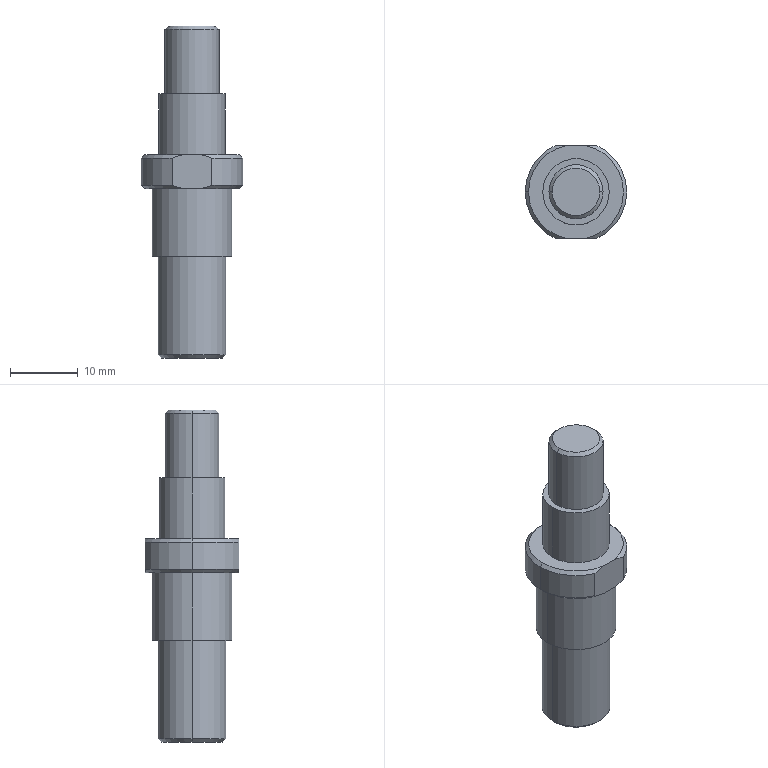Part | SolidWorks | features ICE 5, Chamfer 1, Extrusion 1 | 1 solid | 29 faces | box 15 x 13.8 x 49 mm | volume 4297 mm3 | cylinder 11 | cone 10 | plane 8 | commonest cylinder face diameters 15 x3 8 x2 9.8 x2 10 x2 11.8 x2
STEP:
#1=CARTESIAN_POINT('',(-4.5,0.,-24.5));
#2=VERTEX_POINT('',#1);
#3=CARTESIAN_POINT('',(4.5,0.,-24.5));
#4=VERTEX_POINT('',#3);
#5=CARTESIAN_POINT('',(0.,0.,-24.5));
#6=DIRECTION('',(0.,0.,-1.));
#7=DIRECTION('',(1.,0.,0.));
#8=AXIS2_PLACEMENT_3D('',#5,#6,#7);
#9=CIRCLE('',#8,4.5);
#10=EDGE_CURVE('',#2,#4,#9,.T.);
#11=ORIENTED_EDGE('',*,*,#10,.F.);
#12=CARTESIAN_POINT('',(-5.,0.,-24.));
#13=VERTEX_POINT('',#12);
#14=CARTESIAN_POINT('',(-4.5,0.,-24.5));
#15=DIRECTION('',(-0.7071,0.,0.7071));
#16=VECTOR('',#15,1000.);
#17=LINE('',#14,#16);
#18=EDGE_CURVE('',#2,#13,#17,.T.);
#19=ORIENTED_EDGE('',*,*,#18,.T.);
#20=CARTESIAN_POINT('',(5.,0.,-24.));
#21=VERTEX_POINT('',#20);
#22=CARTESIAN_POINT('',(0.,0.,-24.));
#23=DIRECTION('',(0.,0.,1.));
#24=DIRECTION('',(1.,0.,0.));
#25=AXIS2_PLACEMENT_3D('',#22,#23,#24);
#26=CIRCLE('',#25,5.);
#27=EDGE_CURVE('',#21,#13,#26,.T.);
#28=ORIENTED_EDGE('',*,*,#27,.F.);
#29=CARTESIAN_POINT('',(4.5,0.,-24.5));
#30=DIRECTION('',(0.7071,0.,0.7071));
#31=VECTOR('',#30,1000.);
#32=LINE('',#29,#31);
#33=EDGE_CURVE('',#4,#21,#32,.T.);
#34=ORIENTED_EDGE('',*,*,#33,.F.);
#35=EDGE_LOOP('',(#11,#19,#28,#34));
#36=FACE_OUTER_BOUND('',#35,.T.);
#37=CARTESIAN_POINT('',(0.,0.,-24.5));
#38=DIRECTION('',(0.,0.,1.));
#39=DIRECTION('',(1.,0.,0.));
#40=AXIS2_PLACEMENT_3D('',#37,#38,#39);
#41=CONICAL_SURFACE('',#40,4.5,0.7854);
#42=ADVANCED_FACE('',(#36),#41,.T.);
#43=CARTESIAN_POINT('',(3.5,0.,24.5));
#44=VERTEX_POINT('',#43);
#45=CARTESIAN_POINT('',(-3.5,0.,24.5));
#46=VERTEX_POINT('',#45);
#47=CARTESIAN_POINT('',(0.,0.,24.5));
#48=DIRECTION('',(0.,0.,1.));
#49=DIRECTION('',(1.,0.,0.));
#50=AXIS2_PLACEMENT_3D('',#47,#48,#49);
#51=CIRCLE('',#50,3.5);
#52=EDGE_CURVE('',#44,#46,#51,.T.);
#53=ORIENTED_EDGE('',*,*,#52,.F.);
#54=CARTESIAN_POINT('',(4.,0.,24.));
#55=VERTEX_POINT('',#54);
#56=CARTESIAN_POINT('',(3.5,0.,24.5));
#57=DIRECTION('',(0.7071,0.,-0.7071));
#58=VECTOR('',#57,1000.);
#59=LINE('',#56,#58);
#60=EDGE_CURVE('',#44,#55,#59,.T.);
#61=ORIENTED_EDGE('',*,*,#60,.T.);
#62=CARTESIAN_POINT('',(-4.,0.,24.));
#63=VERTEX_POINT('',#62);
#64=CARTESIAN_POINT('',(0.,0.,24.));
#65=DIRECTION('',(0.,0.,-1.));
#66=DIRECTION('',(1.,0.,0.));
#67=AXIS2_PLACEMENT_3D('',#64,#65,#66);
#68=CIRCLE('',#67,4.);
#69=EDGE_CURVE('',#63,#55,#68,.T.);
#70=ORIENTED_EDGE('',*,*,#69,.F.);
#71=CARTESIAN_POINT('',(-3.5,0.,24.5));
#72=DIRECTION('',(-0.7071,0.,-0.7071));
#73=VECTOR('',#72,1000.);
#74=LINE('',#71,#73);
#75=EDGE_CURVE('',#46,#63,#74,.T.);
#76=ORIENTED_EDGE('',*,*,#75,.F.);
#77=EDGE_LOOP('',(#53,#61,#70,#76));
#78=FACE_OUTER_BOUND('',#77,.T.);
#79=CARTESIAN_POINT('',(0.,0.,24.5));
#80=DIRECTION('',(0.,0.,-1.));
#81=DIRECTION('',(-1.,0.,0.));
#82=AXIS2_PLACEMENT_3D('',#79,#80,#81);
#83=CONICAL_SURFACE('',#82,3.5,0.7854);
#84=ADVANCED_FACE('',(#78),#83,.T.);
#85=CARTESIAN_POINT('',(-7.,0.,5.5));
#86=VERTEX_POINT('',#85);
#87=CARTESIAN_POINT('',(-1.179,-6.9,5.5));
#88=VERTEX_POINT('',#87);
#89=CARTESIAN_POINT('',(0.,0.,5.5));
#90=DIRECTION('',(0.,0.,1.));
#91=DIRECTION('',(1.,0.,0.));
#92=AXIS2_PLACEMENT_3D('',#89,#90,#91);
#93=CIRCLE('',#92,7.);
#94=EDGE_CURVE('',#86,#88,#93,.T.);
#95=ORIENTED_EDGE('',*,*,#94,.F.);
#96=CARTESIAN_POINT('',(-7.5,0.,5.));
#97=VERTEX_POINT('',#96);
#98=CARTESIAN_POINT('',(-7.,0.,5.5));
#99=DIRECTION('',(-0.7071,0.,-0.7071));
#100=VECTOR('',#99,1000.);
#101=LINE('',#98,#100);
#102=EDGE_CURVE('',#86,#97,#101,.T.);
#103=ORIENTED_EDGE('',*,*,#102,.T.);
#104=CARTESIAN_POINT('',(-2.939,-6.9,5.));
#105=VERTEX_POINT('',#104);
#106=CARTESIAN_POINT('',(0.,0.,5.));
#107=DIRECTION('',(0.,0.,-1.));
#108=DIRECTION('',(1.,0.,0.));
#109=AXIS2_PLACEMENT_3D('',#106,#107,#108);
#110=CIRCLE('',#109,7.5);
#111=EDGE_CURVE('',#105,#97,#110,.T.);
#112=ORIENTED_EDGE('',*,*,#111,.F.);
#113=CARTESIAN_POINT('',(-1.179,-6.9,5.5));
#114=CARTESIAN_POINT('',(-1.782,-6.9,5.398));
#115=CARTESIAN_POINT('',(-2.367,-6.9,5.224));
#116=CARTESIAN_POINT('',(-2.939,-6.9,5.));
#117=B_SPLINE_CURVE_WITH_KNOTS('',3,(#113,#114,#115,#116),.UNSPECIFIED.,.F.,.F.,(4,4),(0.01931,0.02115),.UNSPECIFIED.);
#118=EDGE_CURVE('',#88,#105,#117,.T.);
#119=ORIENTED_EDGE('',*,*,#118,.F.);
#120=EDGE_LOOP('',(#95,#103,#112,#119));
#121=FACE_OUTER_BOUND('',#120,.T.);
#122=CARTESIAN_POINT('',(0.,0.,5.5));
#123=DIRECTION('',(0.,0.,-1.));
#124=DIRECTION('',(-1.,0.,0.));
#125=AXIS2_PLACEMENT_3D('',#122,#123,#124);
#126=CONICAL_SURFACE('',#125,7.,0.7854);
#127=ADVANCED_FACE('',(#121),#126,.T.);
#128=CARTESIAN_POINT('',(7.,0.,0.5));
#129=VERTEX_POINT('',#128);
#130=CARTESIAN_POINT('',(1.179,-6.9,0.5));
#131=VERTEX_POINT('',#130);
#132=CARTESIAN_POINT('',(0.,0.,0.5));
#133=DIRECTION('',(0.,0.,-1.));
#134=DIRECTION('',(-1.,0.,0.));
#135=AXIS2_PLACEMENT_3D('',#132,#133,#134);
#136=CIRCLE('',#135,7.);
#137=EDGE_CURVE('',#129,#131,#136,.T.);
#138=ORIENTED_EDGE('',*,*,#137,.F.);
#139=CARTESIAN_POINT('',(7.5,0.,1.));
#140=VERTEX_POINT('',#139);
#141=CARTESIAN_POINT('',(7.,0.,0.5));
#142=DIRECTION('',(0.7071,0.,0.7071));
#143=VECTOR('',#142,1000.);
#144=LINE('',#141,#143);
#145=EDGE_CURVE('',#129,#140,#144,.T.);
#146=ORIENTED_EDGE('',*,*,#145,.T.);
#147=CARTESIAN_POINT('',(2.939,-6.9,1.));
#148=VERTEX_POINT('',#147);
#149=CARTESIAN_POINT('',(0.,0.,1.));
#150=DIRECTION('',(0.,0.,1.));
#151=DIRECTION('',(-1.,0.,0.));
#152=AXIS2_PLACEMENT_3D('',#149,#150,#151);
#153=CIRCLE('',#152,7.5);
#154=EDGE_CURVE('',#148,#140,#153,.T.);
#155=ORIENTED_EDGE('',*,*,#154,.F.);
#156=CARTESIAN_POINT('',(1.179,-6.9,0.5));
#157=CARTESIAN_POINT('',(1.782,-6.9,0.6016));
#158=CARTESIAN_POINT('',(2.367,-6.9,0.7758));
#159=CARTESIAN_POINT('',(2.939,-6.9,1.));
#160=B_SPLINE_CURVE_WITH_KNOTS('',3,(#156,#157,#158,#159),.UNSPECIFIED.,.F.,.F.,(4,4),(0.01931,0.02115),.UNSPECIFIED.);
#161=EDGE_CURVE('',#131,#148,#160,.T.);
#162=ORIENTED_EDGE('',*,*,#161,.F.);
#163=EDGE_LOOP('',(#138,#146,#155,#162));
#164=FACE_OUTER_BOUND('',#163,.T.);
#165=CARTESIAN_POINT('',(0.,0.,0.5));
#166=DIRECTION('',(0.,0.,1.));
#167=DIRECTION('',(1.,0.,0.));
#168=AXIS2_PLACEMENT_3D('',#165,#166,#167);
#169=CONICAL_SURFACE('',#168,7.,0.7854);
#170=ADVANCED_FACE('',(#164),#169,.T.);
#171=CARTESIAN_POINT('',(-5.,0.,-9.5));
#172=VERTEX_POINT('',#171);
#173=CARTESIAN_POINT('',(5.,0.,-9.5));
#174=VERTEX_POINT('',#173);
#175=CARTESIAN_POINT('',(0.,0.,-9.5));
#176=DIRECTION('',(0.,0.,-1.));
#177=DIRECTION('',(-1.,0.,0.));
#178=AXIS2_PLACEMENT_3D('',#175,#176,#177);
#179=CIRCLE('',#178,5.);
#180=EDGE_CURVE('',#172,#174,#179,.T.);
#181=ORIENTED_EDGE('',*,*,#180,.T.);
#182=CARTESIAN_POINT('',(5.,0.,-9.5));
#183=DIRECTION('',(0.,0.,-1.));
#184=VECTOR('',#183,1000.);
#185=LINE('',#182,#184);
#186=EDGE_CURVE('',#174,#21,#185,.T.);
#187=ORIENTED_EDGE('',*,*,#186,.T.);
#188=ORIENTED_EDGE('',*,*,#27,.T.);
#189=CARTESIAN_POINT('',(-5.,0.,-9.5));
#190=DIRECTION('',(0.,0.,-1.));
#191=VECTOR('',#190,1000.);
#192=LINE('',#189,#191);
#193=EDGE_CURVE('',#172,#13,#192,.T.);
#194=ORIENTED_EDGE('',*,*,#193,.F.);
#195=EDGE_LOOP('',(#181,#187,#188,#194));
#196=FACE_OUTER_BOUND('',#195,.T.);
#197=CARTESIAN_POINT('',(0.,0.,-9.5));
#198=DIRECTION('',(0.,0.,-1.));
#199=DIRECTION('',(-1.,0.,0.));
#200=AXIS2_PLACEMENT_3D('',#197,#198,#199);
#201=CYLINDRICAL_SURFACE('',#200,5.);
#202=ADVANCED_FACE('',(#196),#201,.T.);
#203=CARTESIAN_POINT('',(4.,0.,14.5));
#204=VERTEX_POINT('',#203);
#205=CARTESIAN_POINT('',(-4.,0.,14.5));
#206=VERTEX_POINT('',#205);
#207=CARTESIAN_POINT('',(0.,0.,14.5));
#208=DIRECTION('',(0.,0.,1.));
#209=DIRECTION('',(1.,0.,0.));
#210=AXIS2_PLACEMENT_3D('',#207,#208,#209);
#211=CIRCLE('',#210,4.);
#212=EDGE_CURVE('',#204,#206,#211,.T.);
#213=ORIENTED_EDGE('',*,*,#212,.T.);
#214=CARTESIAN_POINT('',(-4.,0.,14.5));
#215=DIRECTION('',(0.,0.,1.));
#216=VECTOR('',#215,1000.);
#217=LINE('',#214,#216);
#218=EDGE_CURVE('',#206,#63,#217,.T.);
#219=ORIENTED_EDGE('',*,*,#218,.T.);
#220=ORIENTED_EDGE('',*,*,#69,.T.);
#221=CARTESIAN_POINT('',(4.,0.,14.5));
#222=DIRECTION('',(0.,0.,1.));
#223=VECTOR('',#222,1000.);
#224=LINE('',#221,#223);
#225=EDGE_CURVE('',#204,#55,#224,.T.);
#226=ORIENTED_EDGE('',*,*,#225,.F.);
#227=EDGE_LOOP('',(#213,#219,#220,#226));
#228=FACE_OUTER_BOUND('',#227,.T.);
#229=CARTESIAN_POINT('',(0.,0.,14.5));
#230=DIRECTION('',(0.,0.,1.));
#231=DIRECTION('',(1.,0.,0.));
#232=AXIS2_PLACEMENT_3D('',#229,#230,#231);
#233=CYLINDRICAL_SURFACE('',#232,4.);
#234=ADVANCED_FACE('',(#228),#233,.T.);
#235=CARTESIAN_POINT('',(4.9,0.,5.5));
#236=VERTEX_POINT('',#235);
#237=CARTESIAN_POINT('',(-4.9,0.,5.5));
#238=VERTEX_POINT('',#237);
#239=CARTESIAN_POINT('',(0.,0.,5.5));
#240=DIRECTION('',(0.,0.,1.));
#241=DIRECTION('',(1.,0.,0.));
#242=AXIS2_PLACEMENT_3D('',#239,#240,#241);
#243=CIRCLE('',#242,4.9);
#244=EDGE_CURVE('',#236,#238,#243,.T.);
#245=ORIENTED_EDGE('',*,*,#244,.T.);
#246=CARTESIAN_POINT('',(-4.9,0.,14.5));
#247=VERTEX_POINT('',#246);
#248=CARTESIAN_POINT('',(-4.9,0.,5.5));
#249=DIRECTION('',(0.,0.,1.));
#250=VECTOR('',#249,1000.);
#251=LINE('',#248,#250);
#252=EDGE_CURVE('',#238,#247,#251,.T.);
#253=ORIENTED_EDGE('',*,*,#252,.T.);
#254=CARTESIAN_POINT('',(4.9,0.,14.5));
#255=VERTEX_POINT('',#254);
#256=CARTESIAN_POINT('',(0.,0.,14.5));
#257=DIRECTION('',(0.,0.,-1.));
#258=DIRECTION('',(1.,0.,0.));
#259=AXIS2_PLACEMENT_3D('',#256,#257,#258);
#260=CIRCLE('',#259,4.9);
#261=EDGE_CURVE('',#247,#255,#260,.T.);
#262=ORIENTED_EDGE('',*,*,#261,.T.);
#263=CARTESIAN_POINT('',(4.9,0.,5.5));
#264=DIRECTION('',(0.,0.,1.));
#265=VECTOR('',#264,1000.);
#266=LINE('',#263,#265);
#267=EDGE_CURVE('',#236,#255,#266,.T.);
#268=ORIENTED_EDGE('',*,*,#267,.F.);
#269=EDGE_LOOP('',(#245,#253,#262,#268));
#270=FACE_OUTER_BOUND('',#269,.T.);
#271=CARTESIAN_POINT('',(0.,0.,5.5));
#272=DIRECTION('',(0.,0.,1.));
#273=DIRECTION('',(1.,0.,0.));
#274=AXIS2_PLACEMENT_3D('',#271,#272,#273);
#275=CYLINDRICAL_SURFACE('',#274,4.9);
#276=ADVANCED_FACE('',(#270),#275,.T.);
#277=ORIENTED_EDGE('',*,*,#111,.T.);
#278=CARTESIAN_POINT('',(-7.5,0.,1.));
#279=VERTEX_POINT('',#278);
#280=CARTESIAN_POINT('',(-7.5,0.,24.5));
#281=DIRECTION('',(0.,0.,-1.));
#282=VECTOR('',#281,1000.);
#283=LINE('',#280,#282);
#284=EDGE_CURVE('',#97,#279,#283,.T.);
#285=ORIENTED_EDGE('',*,*,#284,.T.);
#286=CARTESIAN_POINT('',(-2.939,-6.9,1.));
#287=VERTEX_POINT('',#286);
#288=CARTESIAN_POINT('',(0.,0.,1.));
#289=DIRECTION('',(0.,0.,1.));
#290=DIRECTION('',(-1.,0.,0.));
#291=AXIS2_PLACEMENT_3D('',#288,#289,#290);
#292=CIRCLE('',#291,7.5);
#293=EDGE_CURVE('',#279,#287,#292,.T.);
#294=ORIENTED_EDGE('',*,*,#293,.T.);
#295=CARTESIAN_POINT('',(-2.939,-6.9,24.5));
#296=DIRECTION('',(0.,0.,1.));
#297=VECTOR('',#296,1000.);
#298=LINE('',#295,#297);
#299=EDGE_CURVE('',#287,#105,#298,.T.);
#300=ORIENTED_EDGE('',*,*,#299,.T.);
#301=EDGE_LOOP('',(#277,#285,#294,#300));
#302=FACE_OUTER_BOUND('',#301,.T.);
#303=CARTESIAN_POINT('',(0.,0.,24.5));
#304=DIRECTION('',(0.,0.,-1.));
#305=DIRECTION('',(-1.,0.,0.));
#306=AXIS2_PLACEMENT_3D('',#303,#304,#305);
#307=CYLINDRICAL_SURFACE('',#306,7.5);
#308=ADVANCED_FACE('',(#302),#307,.T.);
#309=CARTESIAN_POINT('',(-5.9,0.,0.5));
#310=VERTEX_POINT('',#309);
#311=CARTESIAN_POINT('',(5.9,0.,0.5));
#312=VERTEX_POINT('',#311);
#313=CARTESIAN_POINT('',(0.,0.,0.5));
#314=DIRECTION('',(0.,0.,-1.));
#315=DIRECTION('',(-1.,0.,0.));
#316=AXIS2_PLACEMENT_3D('',#313,#314,#315);
#317=CIRCLE('',#316,5.9);
#318=EDGE_CURVE('',#310,#312,#317,.T.);
#319=ORIENTED_EDGE('',*,*,#318,.T.);
#320=CARTESIAN_POINT('',(5.9,0.,-9.5));
#321=VERTEX_POINT('',#320);
#322=CARTESIAN_POINT('',(5.9,0.,0.5));
#323=DIRECTION('',(0.,0.,-1.));
#324=VECTOR('',#323,1000.);
#325=LINE('',#322,#324);
#326=EDGE_CURVE('',#312,#321,#325,.T.);
#327=ORIENTED_EDGE('',*,*,#326,.T.);
#328=CARTESIAN_POINT('',(-5.9,0.,-9.5));
#329=VERTEX_POINT('',#328);
#330=CARTESIAN_POINT('',(0.,0.,-9.5));
#331=DIRECTION('',(0.,0.,1.));
#332=DIRECTION('',(-1.,0.,0.));
#333=AXIS2_PLACEMENT_3D('',#330,#331,#332);
#334=CIRCLE('',#333,5.9);
#335=EDGE_CURVE('',#321,#329,#334,.T.);
#336=ORIENTED_EDGE('',*,*,#335,.T.);
#337=CARTESIAN_POINT('',(-5.9,0.,0.5));
#338=DIRECTION('',(0.,0.,-1.));
#339=VECTOR('',#338,1000.);
#340=LINE('',#337,#339);
#341=EDGE_CURVE('',#310,#329,#340,.T.);
#342=ORIENTED_EDGE('',*,*,#341,.F.);
#343=EDGE_LOOP('',(#319,#327,#336,#342));
#344=FACE_OUTER_BOUND('',#343,.T.);
#345=CARTESIAN_POINT('',(0.,0.,0.5));
#346=DIRECTION('',(0.,0.,-1.));
#347=DIRECTION('',(-1.,0.,0.));
#348=AXIS2_PLACEMENT_3D('',#345,#346,#347);
#349=CYLINDRICAL_SURFACE('',#348,5.9);
#350=ADVANCED_FACE('',(#344),#349,.T.);
#351=CARTESIAN_POINT('',(2.939,6.9,5.));
#352=VERTEX_POINT('',#351);
#353=CARTESIAN_POINT('',(2.939,-6.9,5.));
#354=VERTEX_POINT('',#353);
#355=CARTESIAN_POINT('',(0.,0.,5.));
#356=DIRECTION('',(0.,0.,-1.));
#357=DIRECTION('',(1.,0.,0.));
#358=AXIS2_PLACEMENT_3D('',#355,#356,#357);
#359=CIRCLE('',#358,7.5);
#360=EDGE_CURVE('',#352,#354,#359,.T.);
#361=ORIENTED_EDGE('',*,*,#360,.T.);
#362=CARTESIAN_POINT('',(2.939,-6.9,24.5));
#363=DIRECTION('',(0.,0.,-1.));
#364=VECTOR('',#363,1000.);
#365=LINE('',#362,#364);
#366=EDGE_CURVE('',#354,#148,#365,.T.);
#367=ORIENTED_EDGE('',*,*,#366,.T.);
#368=ORIENTED_EDGE('',*,*,#154,.T.);
#369=CARTESIAN_POINT('',(2.939,6.9,1.));
#370=VERTEX_POINT('',#369);
#371=CARTESIAN_POINT('',(0.,0.,1.));
#372=DIRECTION('',(0.,0.,1.));
#373=DIRECTION('',(-1.,0.,0.));
#374=AXIS2_PLACEMENT_3D('',#371,#372,#373);
#375=CIRCLE('',#374,7.5);
#376=EDGE_CURVE('',#140,#370,#375,.T.);
#377=ORIENTED_EDGE('',*,*,#376,.T.);
#378=CARTESIAN_POINT('',(2.939,6.9,24.5));
#379=DIRECTION('',(0.,0.,1.));
#380=VECTOR('',#379,1000.);
#381=LINE('',#378,#380);
#382=EDGE_CURVE('',#370,#352,#381,.T.);
#383=ORIENTED_EDGE('',*,*,#382,.T.);
#384=EDGE_LOOP('',(#361,#367,#368,#377,#383));
#385=FACE_OUTER_BOUND('',#384,.T.);
#386=CARTESIAN_POINT('',(0.,0.,24.5));
#387=DIRECTION('',(0.,0.,-1.));
#388=DIRECTION('',(-1.,0.,0.));
#389=AXIS2_PLACEMENT_3D('',#386,#387,#388);
#390=CYLINDRICAL_SURFACE('',#389,7.5);
#391=ADVANCED_FACE('',(#385),#390,.T.);
#392=CARTESIAN_POINT('',(-1.179,-6.9,0.5));
#393=VERTEX_POINT('',#392);
#394=CARTESIAN_POINT('',(-2.939,-6.9,1.));
#395=CARTESIAN_POINT('',(-2.656,-6.9,0.889));
#396=CARTESIAN_POINT('',(-2.368,-6.9,0.7896));
#397=CARTESIAN_POINT('',(-1.78,-6.9,0.6203));
#398=CARTESIAN_POINT('',(-1.479,-6.9,0.5506));
#399=CARTESIAN_POINT('',(-1.179,-6.9,0.5));
#400=B_SPLINE_CURVE_WITH_KNOTS('',3,(#394,#395,#396,#397,#398,#399),.UNSPECIFIED.,.F.,.F.,(4,2,4),(0.01512,0.01603,0.01694),.UNSPECIFIED.);
#401=EDGE_CURVE('',#287,#393,#400,.T.);
#402=ORIENTED_EDGE('',*,*,#401,.F.);
#403=ORIENTED_EDGE('',*,*,#293,.F.);
#404=CARTESIAN_POINT('',(-2.939,6.9,1.));
#405=VERTEX_POINT('',#404);
#406=CARTESIAN_POINT('',(0.,0.,1.));
#407=DIRECTION('',(0.,0.,1.));
#408=DIRECTION('',(-1.,0.,0.));
#409=AXIS2_PLACEMENT_3D('',#406,#407,#408);
#410=CIRCLE('',#409,7.5);
#411=EDGE_CURVE('',#405,#279,#410,.T.);
#412=ORIENTED_EDGE('',*,*,#411,.F.);
#413=CARTESIAN_POINT('',(-1.179,6.9,0.5));
#414=VERTEX_POINT('',#413);
#415=CARTESIAN_POINT('',(-1.179,6.9,0.5));
#416=CARTESIAN_POINT('',(-1.782,6.9,0.6016));
#417=CARTESIAN_POINT('',(-2.367,6.9,0.7758));
#418=CARTESIAN_POINT('',(-2.939,6.9,1.));
#419=B_SPLINE_CURVE_WITH_KNOTS('',3,(#415,#416,#417,#418),.UNSPECIFIED.,.F.,.F.,(4,4),(0.01931,0.02115),.UNSPECIFIED.);
#420=EDGE_CURVE('',#414,#405,#419,.T.);
#421=ORIENTED_EDGE('',*,*,#420,.F.);
#422=CARTESIAN_POINT('',(0.,0.,0.5));
#423=DIRECTION('',(0.,0.,-1.));
#424=DIRECTION('',(-1.,0.,0.));
#425=AXIS2_PLACEMENT_3D('',#422,#423,#424);
#426=CIRCLE('',#425,7.);
#427=EDGE_CURVE('',#393,#414,#426,.T.);
#428=ORIENTED_EDGE('',*,*,#427,.F.);
#429=EDGE_LOOP('',(#402,#403,#412,#421,#428));
#430=FACE_OUTER_BOUND('',#429,.T.);
#431=CARTESIAN_POINT('',(0.,0.,0.5));
#432=DIRECTION('',(0.,0.,1.));
#433=DIRECTION('',(1.,0.,0.));
#434=AXIS2_PLACEMENT_3D('',#431,#432,#433);
#435=CONICAL_SURFACE('',#434,7.,0.7854);
#436=ADVANCED_FACE('',(#430),#435,.T.);
#437=CARTESIAN_POINT('',(1.179,-6.9,5.5));
#438=VERTEX_POINT('',#437);
#439=CARTESIAN_POINT('',(2.939,-6.9,5.));
#440=CARTESIAN_POINT('',(2.656,-6.9,5.111));
#441=CARTESIAN_POINT('',(2.368,-6.9,5.21));
#442=CARTESIAN_POINT('',(1.78,-6.9,5.38));
#443=CARTESIAN_POINT('',(1.479,-6.9,5.449));
#444=CARTESIAN_POINT('',(1.179,-6.9,5.5));
#445=B_SPLINE_CURVE_WITH_KNOTS('',3,(#439,#440,#441,#442,#443,#444),.UNSPECIFIED.,.F.,.F.,(4,2,4),(0.01512,0.01603,0.01694),.UNSPECIFIED.);
#446=EDGE_CURVE('',#354,#438,#445,.T.);
#447=ORIENTED_EDGE('',*,*,#446,.F.);
#448=ORIENTED_EDGE('',*,*,#360,.F.);
#449=CARTESIAN_POINT('',(1.179,6.9,5.5));
#450=VERTEX_POINT('',#449);
#451=CARTESIAN_POINT('',(1.179,6.9,5.5));
#452=CARTESIAN_POINT('',(1.782,6.9,5.398));
#453=CARTESIAN_POINT('',(2.367,6.9,5.224));
#454=CARTESIAN_POINT('',(2.939,6.9,5.));
#455=B_SPLINE_CURVE_WITH_KNOTS('',3,(#451,#452,#453,#454),.UNSPECIFIED.,.F.,.F.,(4,4),(0.01931,0.02115),.UNSPECIFIED.);
#456=EDGE_CURVE('',#450,#352,#455,.T.);
#457=ORIENTED_EDGE('',*,*,#456,.F.);
#458=CARTESIAN_POINT('',(0.,0.,5.5));
#459=DIRECTION('',(0.,0.,1.));
#460=DIRECTION('',(1.,0.,0.));
#461=AXIS2_PLACEMENT_3D('',#458,#459,#460);
#462=CIRCLE('',#461,7.);
#463=EDGE_CURVE('',#438,#450,#462,.T.);
#464=ORIENTED_EDGE('',*,*,#463,.F.);
#465=EDGE_LOOP('',(#447,#448,#457,#464));
#466=FACE_OUTER_BOUND('',#465,.T.);
#467=CARTESIAN_POINT('',(0.,0.,5.5));
#468=DIRECTION('',(0.,0.,-1.));
#469=DIRECTION('',(-1.,0.,0.));
#470=AXIS2_PLACEMENT_3D('',#467,#468,#469);
#471=CONICAL_SURFACE('',#470,7.,0.7854);
#472=ADVANCED_FACE('',(#466),#471,.T.);
#473=ORIENTED_EDGE('',*,*,#326,.F.);
#474=CARTESIAN_POINT('',(0.,0.,0.5));
#475=DIRECTION('',(0.,0.,-1.));
#476=DIRECTION('',(-1.,0.,0.));
#477=AXIS2_PLACEMENT_3D('',#474,#475,#476);
#478=CIRCLE('',#477,5.9);
#479=EDGE_CURVE('',#312,#310,#478,.T.);
#480=ORIENTED_EDGE('',*,*,#479,.T.);
#481=ORIENTED_EDGE('',*,*,#341,.T.);
#482=CARTESIAN_POINT('',(0.,0.,-9.5));
#483=DIRECTION('',(0.,0.,1.));
#484=DIRECTION('',(-1.,0.,0.));
#485=AXIS2_PLACEMENT_3D('',#482,#483,#484);
#486=CIRCLE('',#485,5.9);
#487=EDGE_CURVE('',#329,#321,#486,.T.);
#488=ORIENTED_EDGE('',*,*,#487,.T.);
#489=EDGE_LOOP('',(#473,#480,#481,#488));
#490=FACE_OUTER_BOUND('',#489,.T.);
#491=CARTESIAN_POINT('',(0.,0.,0.5));
#492=DIRECTION('',(0.,0.,-1.));
#493=DIRECTION('',(-1.,0.,0.));
#494=AXIS2_PLACEMENT_3D('',#491,#492,#493);
#495=CYLINDRICAL_SURFACE('',#494,5.9);
#496=ADVANCED_FACE('',(#490),#495,.T.);
#497=ORIENTED_EDGE('',*,*,#284,.F.);
#498=CARTESIAN_POINT('',(-2.939,6.9,5.));
#499=VERTEX_POINT('',#498);
#500=CARTESIAN_POINT('',(0.,0.,5.));
#501=DIRECTION('',(0.,0.,-1.));
#502=DIRECTION('',(1.,0.,0.));
#503=AXIS2_PLACEMENT_3D('',#500,#501,#502);
#504=CIRCLE('',#503,7.5);
#505=EDGE_CURVE('',#97,#499,#504,.T.);
#506=ORIENTED_EDGE('',*,*,#505,.T.);
#507=CARTESIAN_POINT('',(-2.939,6.9,24.5));
#508=DIRECTION('',(0.,0.,-1.));
#509=VECTOR('',#508,1000.);
#510=LINE('',#507,#509);
#511=EDGE_CURVE('',#499,#405,#510,.T.);
#512=ORIENTED_EDGE('',*,*,#511,.T.);
#513=ORIENTED_EDGE('',*,*,#411,.T.);
#514=EDGE_LOOP('',(#497,#506,#512,#513));
#515=FACE_OUTER_BOUND('',#514,.T.);
#516=CARTESIAN_POINT('',(0.,0.,24.5));
#517=DIRECTION('',(0.,0.,-1.));
#518=DIRECTION('',(-1.,0.,0.));
#519=AXIS2_PLACEMENT_3D('',#516,#517,#518);
#520=CYLINDRICAL_SURFACE('',#519,7.5);
#521=ADVANCED_FACE('',(#515),#520,.T.);
#522=ORIENTED_EDGE('',*,*,#252,.F.);
#523=CARTESIAN_POINT('',(0.,0.,5.5));
#524=DIRECTION('',(0.,0.,1.));
#525=DIRECTION('',(1.,0.,0.));
#526=AXIS2_PLACEMENT_3D('',#523,#524,#525);
#527=CIRCLE('',#526,4.9);
#528=EDGE_CURVE('',#238,#236,#527,.T.);
#529=ORIENTED_EDGE('',*,*,#528,.T.);
#530=ORIENTED_EDGE('',*,*,#267,.T.);
#531=CARTESIAN_POINT('',(0.,0.,14.5));
#532=DIRECTION('',(0.,0.,-1.));
#533=DIRECTION('',(1.,0.,0.));
#534=AXIS2_PLACEMENT_3D('',#531,#532,#533);
#535=CIRCLE('',#534,4.9);
#536=EDGE_CURVE('',#255,#247,#535,.T.);
#537=ORIENTED_EDGE('',*,*,#536,.T.);
#538=EDGE_LOOP('',(#522,#529,#530,#537));
#539=FACE_OUTER_BOUND('',#538,.T.);
#540=CARTESIAN_POINT('',(0.,0.,5.5));
#541=DIRECTION('',(0.,0.,1.));
#542=DIRECTION('',(1.,0.,0.));
#543=AXIS2_PLACEMENT_3D('',#540,#541,#542);
#544=CYLINDRICAL_SURFACE('',#543,4.9);
#545=ADVANCED_FACE('',(#539),#544,.T.);
#546=CARTESIAN_POINT('',(-7.5,-6.9,5.5));
#547=DIRECTION('',(-1.,0.,0.));
#548=VECTOR('',#547,1000.);
#549=LINE('',#546,#548);
#550=EDGE_CURVE('',#438,#88,#549,.T.);
#551=ORIENTED_EDGE('',*,*,#550,.F.);
#552=ORIENTED_EDGE('',*,*,#463,.T.);
#553=CARTESIAN_POINT('',(-1.179,6.9,5.5));
#554=VERTEX_POINT('',#553);
#555=CARTESIAN_POINT('',(-7.5,6.9,5.5));
#556=DIRECTION('',(1.,0.,0.));
#557=VECTOR('',#556,1000.);
#558=LINE('',#555,#557);
#559=EDGE_CURVE('',#554,#450,#558,.T.);
#560=ORIENTED_EDGE('',*,*,#559,.F.);
#561=CARTESIAN_POINT('',(0.,0.,5.5));
#562=DIRECTION('',(0.,0.,1.));
#563=DIRECTION('',(1.,0.,0.));
#564=AXIS2_PLACEMENT_3D('',#561,#562,#563);
#565=CIRCLE('',#564,7.);
#566=EDGE_CURVE('',#554,#86,#565,.T.);
#567=ORIENTED_EDGE('',*,*,#566,.T.);
#568=ORIENTED_EDGE('',*,*,#94,.T.);
#569=EDGE_LOOP('',(#551,#552,#560,#567,#568));
#570=FACE_OUTER_BOUND('',#569,.T.);
#571=ORIENTED_EDGE('',*,*,#244,.F.);
#572=ORIENTED_EDGE('',*,*,#528,.F.);
#573=EDGE_LOOP('',(#571,#572));
#574=FACE_BOUND('',#573,.T.);
#575=CARTESIAN_POINT('',(0.,0.,5.5));
#576=DIRECTION('',(0.,0.,1.));
#577=DIRECTION('',(1.,0.,0.));
#578=AXIS2_PLACEMENT_3D('',#575,#576,#577);
#579=PLANE('',#578);
#580=ADVANCED_FACE('',(#570,#574),#579,.T.);
#581=ORIENTED_EDGE('',*,*,#536,.F.);
#582=ORIENTED_EDGE('',*,*,#261,.F.);
#583=EDGE_LOOP('',(#581,#582));
#584=FACE_OUTER_BOUND('',#583,.T.);
#585=ORIENTED_EDGE('',*,*,#212,.F.);
#586=CARTESIAN_POINT('',(0.,0.,14.5));
#587=DIRECTION('',(0.,0.,1.));
#588=DIRECTION('',(1.,0.,0.));
#589=AXIS2_PLACEMENT_3D('',#586,#587,#588);
#590=CIRCLE('',#589,4.);
#591=EDGE_CURVE('',#206,#204,#590,.T.);
#592=ORIENTED_EDGE('',*,*,#591,.F.);
#593=EDGE_LOOP('',(#585,#592));
#594=FACE_BOUND('',#593,.T.);
#595=CARTESIAN_POINT('',(0.,0.,14.5));
#596=DIRECTION('',(0.,0.,1.));
#597=DIRECTION('',(1.,0.,0.));
#598=AXIS2_PLACEMENT_3D('',#595,#596,#597);
#599=PLANE('',#598);
#600=ADVANCED_FACE('',(#584,#594),#599,.T.);
#601=ORIENTED_EDGE('',*,*,#218,.F.);
#602=ORIENTED_EDGE('',*,*,#591,.T.);
#603=ORIENTED_EDGE('',*,*,#225,.T.);
#604=CARTESIAN_POINT('',(0.,0.,24.));
#605=DIRECTION('',(0.,0.,-1.));
#606=DIRECTION('',(1.,0.,0.));
#607=AXIS2_PLACEMENT_3D('',#604,#605,#606);
#608=CIRCLE('',#607,4.);
#609=EDGE_CURVE('',#55,#63,#608,.T.);
#610=ORIENTED_EDGE('',*,*,#609,.T.);
#611=EDGE_LOOP('',(#601,#602,#603,#610));
#612=FACE_OUTER_BOUND('',#611,.T.);
#613=CARTESIAN_POINT('',(0.,0.,14.5));
#614=DIRECTION('',(0.,0.,1.));
#615=DIRECTION('',(1.,0.,0.));
#616=AXIS2_PLACEMENT_3D('',#613,#614,#615);
#617=CYLINDRICAL_SURFACE('',#616,4.);
#618=ADVANCED_FACE('',(#612),#617,.T.);
#619=CARTESIAN_POINT('',(0.,0.,24.5));
#620=DIRECTION('',(0.,0.,1.));
#621=DIRECTION('',(1.,0.,0.));
#622=AXIS2_PLACEMENT_3D('',#619,#620,#621);
#623=CIRCLE('',#622,3.5);
#624=EDGE_CURVE('',#46,#44,#623,.T.);
#625=ORIENTED_EDGE('',*,*,#624,.T.);
#626=ORIENTED_EDGE('',*,*,#52,.T.);
#627=EDGE_LOOP('',(#625,#626));
#628=FACE_OUTER_BOUND('',#627,.T.);
#629=CARTESIAN_POINT('',(0.,0.,24.5));
#630=DIRECTION('',(0.,0.,1.));
#631=DIRECTION('',(1.,0.,0.));
#632=AXIS2_PLACEMENT_3D('',#629,#630,#631);
#633=PLANE('',#632);
#634=ADVANCED_FACE('',(#628),#633,.T.);
#635=CARTESIAN_POINT('',(0.,-6.9,0.5));
#636=DIRECTION('',(1.,0.,0.));
#637=VECTOR('',#636,1000.);
#638=LINE('',#635,#637);
#639=EDGE_CURVE('',#393,#131,#638,.T.);
#640=ORIENTED_EDGE('',*,*,#639,.F.);
#641=ORIENTED_EDGE('',*,*,#427,.T.);
#642=CARTESIAN_POINT('',(1.179,6.9,0.5));
#643=VERTEX_POINT('',#642);
#644=CARTESIAN_POINT('',(0.,6.9,0.5));
#645=DIRECTION('',(-1.,0.,0.));
#646=VECTOR('',#645,1000.);
#647=LINE('',#644,#646);
#648=EDGE_CURVE('',#643,#414,#647,.T.);
#649=ORIENTED_EDGE('',*,*,#648,.F.);
#650=CARTESIAN_POINT('',(0.,0.,0.5));
#651=DIRECTION('',(0.,0.,-1.));
#652=DIRECTION('',(-1.,0.,0.));
#653=AXIS2_PLACEMENT_3D('',#650,#651,#652);
#654=CIRCLE('',#653,7.);
#655=EDGE_CURVE('',#643,#129,#654,.T.);
#656=ORIENTED_EDGE('',*,*,#655,.T.);
#657=ORIENTED_EDGE('',*,*,#137,.T.);
#658=EDGE_LOOP('',(#640,#641,#649,#656,#657));
#659=FACE_OUTER_BOUND('',#658,.T.);
#660=ORIENTED_EDGE('',*,*,#318,.F.);
#661=ORIENTED_EDGE('',*,*,#479,.F.);
#662=EDGE_LOOP('',(#660,#661));
#663=FACE_BOUND('',#662,.T.);
#664=CARTESIAN_POINT('',(0.,0.,0.5));
#665=DIRECTION('',(0.,0.,-1.));
#666=DIRECTION('',(-1.,0.,0.));
#667=AXIS2_PLACEMENT_3D('',#664,#665,#666);
#668=PLANE('',#667);
#669=ADVANCED_FACE('',(#659,#663),#668,.T.);
#670=ORIENTED_EDGE('',*,*,#487,.F.);
#671=ORIENTED_EDGE('',*,*,#335,.F.);
#672=EDGE_LOOP('',(#670,#671));
#673=FACE_OUTER_BOUND('',#672,.T.);
#674=ORIENTED_EDGE('',*,*,#180,.F.);
#675=CARTESIAN_POINT('',(0.,0.,-9.5));
#676=DIRECTION('',(0.,0.,-1.));
#677=DIRECTION('',(-1.,0.,0.));
#678=AXIS2_PLACEMENT_3D('',#675,#676,#677);
#679=CIRCLE('',#678,5.);
#680=EDGE_CURVE('',#174,#172,#679,.T.);
#681=ORIENTED_EDGE('',*,*,#680,.F.);
#682=EDGE_LOOP('',(#674,#681));
#683=FACE_BOUND('',#682,.T.);
#684=CARTESIAN_POINT('',(0.,0.,-9.5));
#685=DIRECTION('',(0.,0.,-1.));
#686=DIRECTION('',(-1.,0.,0.));
#687=AXIS2_PLACEMENT_3D('',#684,#685,#686);
#688=PLANE('',#687);
#689=ADVANCED_FACE('',(#673,#683),#688,.T.);
#690=ORIENTED_EDGE('',*,*,#186,.F.);
#691=ORIENTED_EDGE('',*,*,#680,.T.);
#692=ORIENTED_EDGE('',*,*,#193,.T.);
#693=CARTESIAN_POINT('',(0.,0.,-24.));
#694=DIRECTION('',(0.,0.,1.));
#695=DIRECTION('',(1.,0.,0.));
#696=AXIS2_PLACEMENT_3D('',#693,#694,#695);
#697=CIRCLE('',#696,5.);
#698=EDGE_CURVE('',#13,#21,#697,.T.);
#699=ORIENTED_EDGE('',*,*,#698,.T.);
#700=EDGE_LOOP('',(#690,#691,#692,#699));
#701=FACE_OUTER_BOUND('',#700,.T.);
#702=CARTESIAN_POINT('',(0.,0.,-9.5));
#703=DIRECTION('',(0.,0.,-1.));
#704=DIRECTION('',(-1.,0.,0.));
#705=AXIS2_PLACEMENT_3D('',#702,#703,#704);
#706=CYLINDRICAL_SURFACE('',#705,5.);
#707=ADVANCED_FACE('',(#701),#706,.T.);
#708=CARTESIAN_POINT('',(0.,0.,-24.5));
#709=DIRECTION('',(0.,0.,-1.));
#710=DIRECTION('',(1.,0.,0.));
#711=AXIS2_PLACEMENT_3D('',#708,#709,#710);
#712=CIRCLE('',#711,4.5);
#713=EDGE_CURVE('',#4,#2,#712,.T.);
#714=ORIENTED_EDGE('',*,*,#713,.T.);
#715=ORIENTED_EDGE('',*,*,#10,.T.);
#716=EDGE_LOOP('',(#714,#715));
#717=FACE_OUTER_BOUND('',#716,.T.);
#718=CARTESIAN_POINT('',(0.,0.,-24.5));
#719=DIRECTION('',(0.,0.,1.));
#720=DIRECTION('',(1.,0.,0.));
#721=AXIS2_PLACEMENT_3D('',#718,#719,#720);
#722=PLANE('',#721);
#723=ADVANCED_FACE('',(#717),#722,.F.);
#724=ORIENTED_EDGE('',*,*,#145,.F.);
#725=ORIENTED_EDGE('',*,*,#655,.F.);
#726=CARTESIAN_POINT('',(2.939,6.9,1.));
#727=CARTESIAN_POINT('',(2.656,6.9,0.889));
#728=CARTESIAN_POINT('',(2.368,6.9,0.7896));
#729=CARTESIAN_POINT('',(1.78,6.9,0.6203));
#730=CARTESIAN_POINT('',(1.479,6.9,0.5506));
#731=CARTESIAN_POINT('',(1.179,6.9,0.5));
#732=B_SPLINE_CURVE_WITH_KNOTS('',3,(#726,#727,#728,#729,#730,#731),.UNSPECIFIED.,.F.,.F.,(4,2,4),(0.01512,0.01603,0.01694),.UNSPECIFIED.);
#733=EDGE_CURVE('',#370,#643,#732,.T.);
#734=ORIENTED_EDGE('',*,*,#733,.F.);
#735=ORIENTED_EDGE('',*,*,#376,.F.);
#736=EDGE_LOOP('',(#724,#725,#734,#735));
#737=FACE_OUTER_BOUND('',#736,.T.);
#738=CARTESIAN_POINT('',(0.,0.,0.5));
#739=DIRECTION('',(0.,0.,1.));
#740=DIRECTION('',(1.,0.,0.));
#741=AXIS2_PLACEMENT_3D('',#738,#739,#740);
#742=CONICAL_SURFACE('',#741,7.,0.7854);
#743=ADVANCED_FACE('',(#737),#742,.T.);
#744=ORIENTED_EDGE('',*,*,#102,.F.);
#745=ORIENTED_EDGE('',*,*,#566,.F.);
#746=CARTESIAN_POINT('',(-2.939,6.9,5.));
#747=CARTESIAN_POINT('',(-2.656,6.9,5.111));
#748=CARTESIAN_POINT('',(-2.368,6.9,5.21));
#749=CARTESIAN_POINT('',(-1.78,6.9,5.38));
#750=CARTESIAN_POINT('',(-1.479,6.9,5.449));
#751=CARTESIAN_POINT('',(-1.179,6.9,5.5));
#752=B_SPLINE_CURVE_WITH_KNOTS('',3,(#746,#747,#748,#749,#750,#751),.UNSPECIFIED.,.F.,.F.,(4,2,4),(0.01512,0.01603,0.01694),.UNSPECIFIED.);
#753=EDGE_CURVE('',#499,#554,#752,.T.);
#754=ORIENTED_EDGE('',*,*,#753,.F.);
#755=ORIENTED_EDGE('',*,*,#505,.F.);
#756=EDGE_LOOP('',(#744,#745,#754,#755));
#757=FACE_OUTER_BOUND('',#756,.T.);
#758=CARTESIAN_POINT('',(0.,0.,5.5));
#759=DIRECTION('',(0.,0.,-1.));
#760=DIRECTION('',(-1.,0.,0.));
#761=AXIS2_PLACEMENT_3D('',#758,#759,#760);
#762=CONICAL_SURFACE('',#761,7.,0.7854);
#763=ADVANCED_FACE('',(#757),#762,.T.);
#764=ORIENTED_EDGE('',*,*,#60,.F.);
#765=ORIENTED_EDGE('',*,*,#624,.F.);
#766=ORIENTED_EDGE('',*,*,#75,.T.);
#767=ORIENTED_EDGE('',*,*,#609,.F.);
#768=EDGE_LOOP('',(#764,#765,#766,#767));
#769=FACE_OUTER_BOUND('',#768,.T.);
#770=CARTESIAN_POINT('',(0.,0.,24.5));
#771=DIRECTION('',(0.,0.,-1.));
#772=DIRECTION('',(-1.,0.,0.));
#773=AXIS2_PLACEMENT_3D('',#770,#771,#772);
#774=CONICAL_SURFACE('',#773,3.5,0.7854);
#775=ADVANCED_FACE('',(#769),#774,.T.);
#776=ORIENTED_EDGE('',*,*,#18,.F.);
#777=ORIENTED_EDGE('',*,*,#713,.F.);
#778=ORIENTED_EDGE('',*,*,#33,.T.);
#779=ORIENTED_EDGE('',*,*,#698,.F.);
#780=EDGE_LOOP('',(#776,#777,#778,#779));
#781=FACE_OUTER_BOUND('',#780,.T.);
#782=CARTESIAN_POINT('',(0.,0.,-24.5));
#783=DIRECTION('',(0.,0.,1.));
#784=DIRECTION('',(1.,0.,0.));
#785=AXIS2_PLACEMENT_3D('',#782,#783,#784);
#786=CONICAL_SURFACE('',#785,4.5,0.7854);
#787=ADVANCED_FACE('',(#781),#786,.T.);
#788=ORIENTED_EDGE('',*,*,#753,.T.);
#789=ORIENTED_EDGE('',*,*,#559,.T.);
#790=ORIENTED_EDGE('',*,*,#456,.T.);
#791=ORIENTED_EDGE('',*,*,#382,.F.);
#792=ORIENTED_EDGE('',*,*,#733,.T.);
#793=ORIENTED_EDGE('',*,*,#648,.T.);
#794=ORIENTED_EDGE('',*,*,#420,.T.);
#795=ORIENTED_EDGE('',*,*,#511,.F.);
#796=EDGE_LOOP('',(#788,#789,#790,#791,#792,#793,#794,#795));
#797=FACE_OUTER_BOUND('',#796,.T.);
#798=CARTESIAN_POINT('',(-7.5,6.9,-9.5));
#799=DIRECTION('',(0.,-1.,0.));
#800=DIRECTION('',(1.,0.,0.));
#801=AXIS2_PLACEMENT_3D('',#798,#799,#800);
#802=PLANE('',#801);
#803=ADVANCED_FACE('',(#797),#802,.F.);
#804=ORIENTED_EDGE('',*,*,#446,.T.);
#805=ORIENTED_EDGE('',*,*,#550,.T.);
#806=ORIENTED_EDGE('',*,*,#118,.T.);
#807=ORIENTED_EDGE('',*,*,#299,.F.);
#808=ORIENTED_EDGE('',*,*,#401,.T.);
#809=ORIENTED_EDGE('',*,*,#639,.T.);
#810=ORIENTED_EDGE('',*,*,#161,.T.);
#811=ORIENTED_EDGE('',*,*,#366,.F.);
#812=EDGE_LOOP('',(#804,#805,#806,#807,#808,#809,#810,#811));
#813=FACE_OUTER_BOUND('',#812,.T.);
#814=CARTESIAN_POINT('',(-7.5,-6.9,-9.5));
#815=DIRECTION('',(0.,1.,0.));
#816=DIRECTION('',(-1.,0.,0.));
#817=AXIS2_PLACEMENT_3D('',#814,#815,#816);
#818=PLANE('',#817);
#819=ADVANCED_FACE('',(#813),#818,.F.);
#820=CLOSED_SHELL('',(#42,#84,#127,#170,#202,#234,#276,#308,#350,#391,#436,#472,#496,#521,#545,#580,#600,#618,#634,#669,#689,#707,#723,#743,#763,#775,#787,#803,#819));
#821=MANIFOLD_SOLID_BREP('',#820);
#822=CARTESIAN_POINT('',(0.,0.,0.));
#823=DIRECTION('',(0.,0.,1.));
#824=DIRECTION('',(1.,0.,0.));
#825=AXIS2_PLACEMENT_3D('',#822,#823,#824);
#826=(LENGTH_UNIT()NAMED_UNIT(*)SI_UNIT(.MILLI.,.METRE.));
#827=UNCERTAINTY_MEASURE_WITH_UNIT(LENGTH_MEASURE(0.00001),#826,'','');
#828=(NAMED_UNIT(*)PLANE_ANGLE_UNIT()SI_UNIT($,.RADIAN.));
#829=(NAMED_UNIT(*)SI_UNIT($,.STERADIAN.)SOLID_ANGLE_UNIT());
#830=(GEOMETRIC_REPRESENTATION_CONTEXT(3)GLOBAL_UNCERTAINTY_ASSIGNED_CONTEXT((#827))GLOBAL_UNIT_ASSIGNED_CONTEXT((#826,#828,#829))REPRESENTATION_CONTEXT('',''));
#831=ADVANCED_BREP_SHAPE_REPRESENTATION('',(#821,#825),#830);